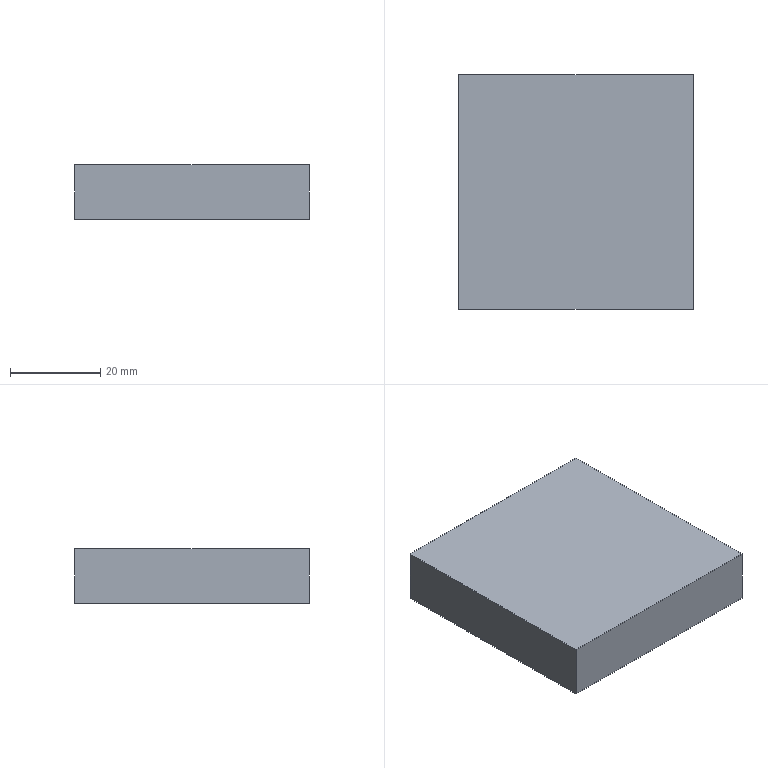NC program | NX | posted with a generic post | part box 52 x 52 x 12 mm
Lines 1 to 18 of 2608:
N10 G17 G21 G94 G90
(PLANAR_MILL , TOOL : D50面刀)
N12 T01 M6
N14 G53
N16 G17 G0 G90 X54.5 Y2.5 S4500 M3
N18 G43 Z30. H1
N20 Z3.
N22 G94 G1 Z0. F800.
N24 X27.5
N26 X-27.5
N28 X-54.5
N30 Z3.
N32 G0 Z30.
N34 M5